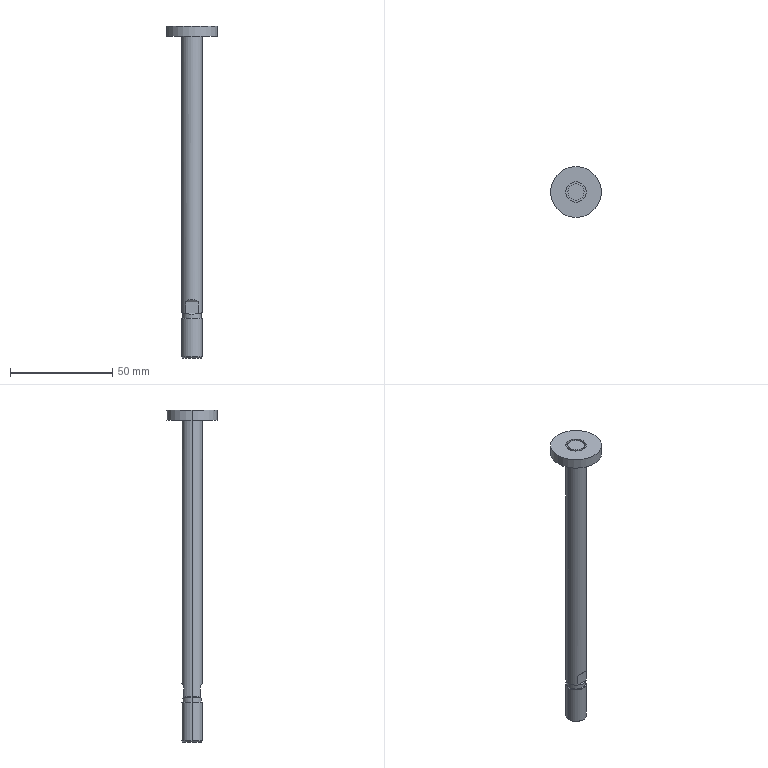Part | STEP file | 0229_Z_Cylinder_CG1DN25-75_3 | 1 solid | 33 faces | box 24.9 x 24.9 x 162.5 mm | volume 14688 mm3 | plane 14 | cylinder 12 | cone 7 | commonest cylinder face diameters 10 x6 8 x2 9.1 x2 24.9 x2